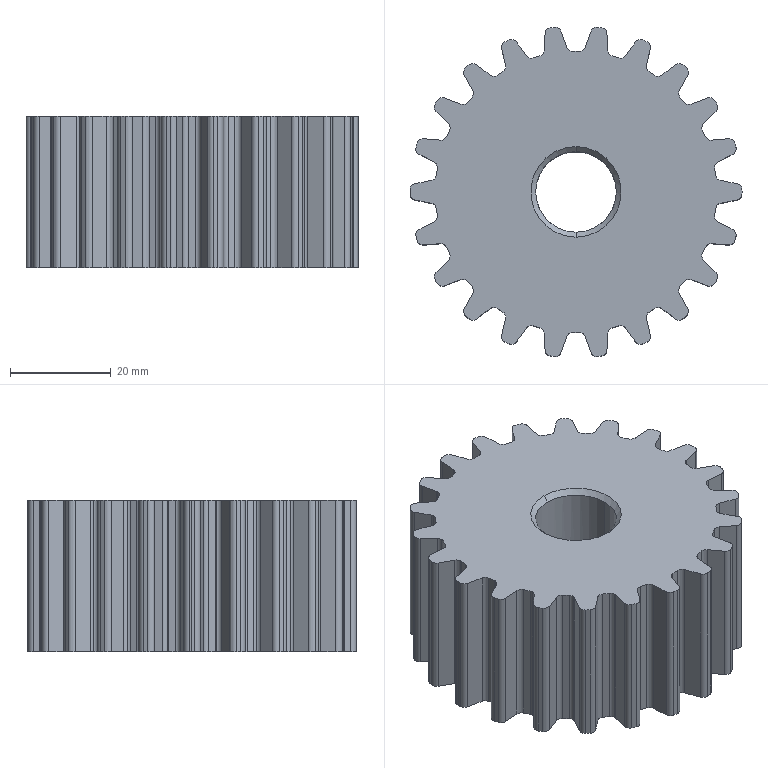Part | STEP file | Timing pulley | 1 solid | 201 faces | box 65.94 x 65.413 x 30 mm | volume 80276 mm3 | cylinder 129 | plane 68 | cone 4 | commonest cylinder face diameters 2.34 x52 2.38 x52 65.94 x23 16 x2